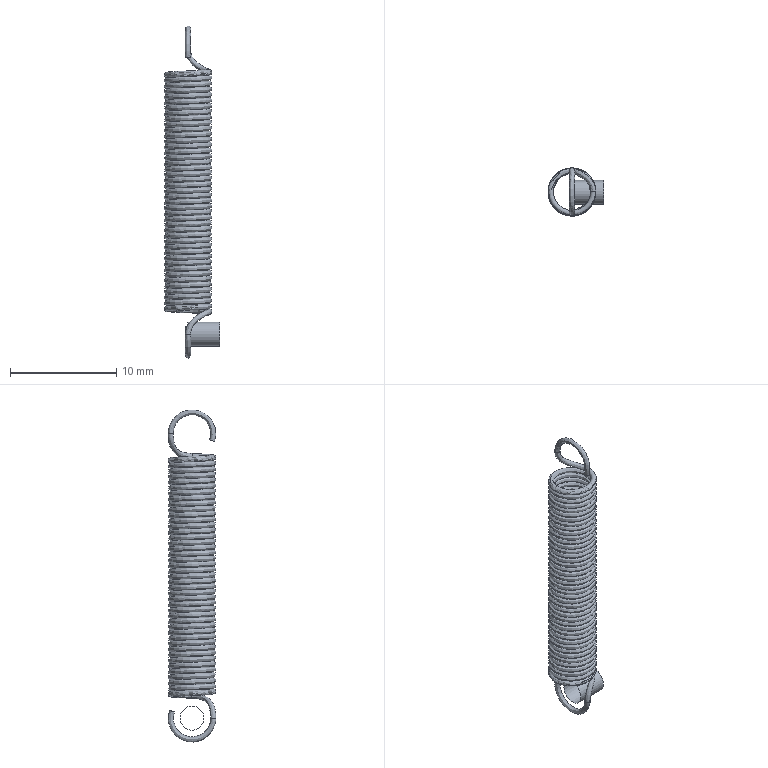Part | NX | features DATUM_CSYS 4, DATUM_AXIS 3, SKETCH 3, BRIDGE_CURVE 2, DATUM_PLANE 2, DATUM_ON_PATH 1, EXTRUDE 1, FLEXIBLE_PART 1, FSET 1, HELIX 1, SKIN 1 | 1 solid | 8 faces | box 5.249 x 4.5 x 31.219 mm | volume 113.865 mm3 | spline 5 | plane 2 | cylinder 1 | commonest cylinder face diameters 2.252 x1